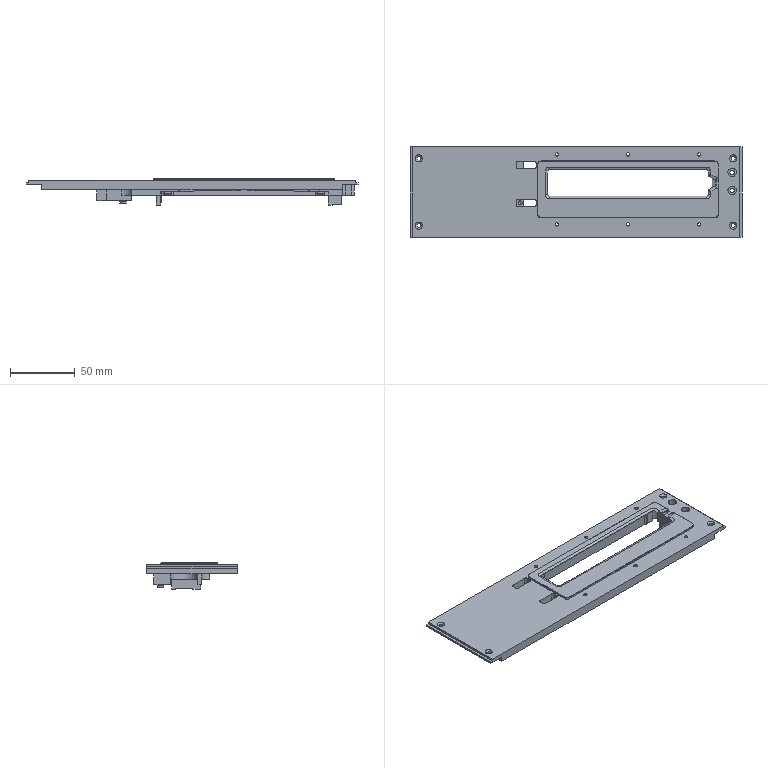NC program | NX | posted with a generic post | part box 256.6 x 70.3 x 20.422 mm
Lines 3316 to 4278 of 23702:
(CAVITY_MILL_COPY , TOOL : D6)
N6624 T06 M6
N6626 G54
N6628 G17 G0 G90 X20.674 Y0.131 S9500 M3
N6630 G43 Z30. H6
N6632 Z-0.118
N6634 G94 G1 Z-1.118 F1000.
N6636 G3 X21.494 Y0.695 R1.
N6638 G2 X21.913 Y1.34 R3. F1800.
N6640 G1 Y2.189
N6642 G3 X21.413 Y3.055 R1.
N6644 G1 X21.313 Y3.113
N6646 Z-0.118
N6648 G0 X20.598 Y-0.536 Z-0.522
N6650 G1 Z-1.522 F1000.
N6652 G3 X21.299 Y0.17 R1.
N6654 G2 X21.509 Y0.726 R3. F1800.
N6656 G1 Y1.349
N6658 G3 X21.009 Y2.215 R1.
N6660 G1 X20.909 Y2.272
N6662 Z-0.522
N6664 G0 X20.598 Y0.633 Z-1.022
N6666 G1 Z-2.022 F1000.
N6668 X20.698 Y0.691
N6670 G3 X21.198 Y1.557 R1.
N6672 G1 Y2.095 F1800.
N6674 G2 X21.057 Y2.607 R3.054
N6676 G3 X20.406 Y3.369 R1.
N6678 G1 Z-1.022
N6680 G0 X20.598 Y0.244 Z-1.522
N6682 G1 Z-2.522 F1000.
N6684 X20.698 Y0.301
N6686 G3 X21.198 Y1.167 R1.
N6688 G1 Y1.851 F1800.
N6690 G2 X20.937 Y2.437 R3.
N6692 G3 X20.2 Y3.106 R1.
N6694 G1 Z-1.522
N6696 G0 X20.598 Y0.244 Z-2.022
N6698 G1 Z-3.022 F1000.
N6700 X20.698 Y0.301
N6702 G3 X21.198 Y1.167 R1.
N6704 G1 Y1.851 F1800.
N6706 G2 X20.937 Y2.437 R3.
N6708 G3 X20.2 Y3.106 R1.
N6710 G1 Z-2.022
N6712 G0 X20.598 Y0.244 Z-2.522
N6714 G1 Z-3.522 F1000.
N6716 X20.698 Y0.301
N6718 G3 X21.198 Y1.167 R1.
N6720 G1 Y1.851 F1800.
N6722 G2 X20.937 Y2.437 R3.
N6724 G3 X20.2 Y3.106 R1.
N6726 G1 Z-2.522
N6728 G0 X20.598 Y0.244 Z-2.988
N6730 G1 Z-3.988 F1000.
N6732 X20.698 Y0.301
N6734 G3 X21.198 Y1.167 R1.
N6736 G1 Y1.851 F1800.
N6738 G2 X20.937 Y2.437 R3.
N6740 G3 X20.2 Y3.106 R1.
N6742 G1 Z-2.988
N6744 G0 X20.598 Y0.244 Z-3.455
N6746 G1 Z-4.455 F1000.
N6748 X20.698 Y0.301
N6750 G3 X21.198 Y1.167 R1.
N6752 G1 Y1.851 F1800.
N6754 G2 X20.937 Y2.437 R3.
N6756 G3 X20.2 Y3.106 R1.
N6758 G1 Z-3.455
N6760 G0 X20.598 Y0.244 Z-3.922
N6762 G1 Z-4.922 F1000.
N6764 X20.698 Y0.301
N6766 G3 X21.198 Y1.167 R1.
N6768 G1 Y1.851 F1800.
N6770 G2 X20.937 Y2.437 R3.
N6772 G3 X20.2 Y3.106 R1.
N6774 G1 Z-3.922
N6776 G0 X20.598 Y0.244 Z-4.388
N6778 G1 Z-5.388 F1000.
N6780 X20.698 Y0.301
N6782 G3 X21.198 Y1.167 R1.
N6784 G1 Y1.851 F1800.
N6786 G2 X20.937 Y2.437 R3.
N6788 G3 X20.2 Y3.106 R1.
N6790 G1 Z-4.388
N6792 G0 X20.598 Y0.244 Z-4.855
N6794 G1 Z-5.855 F1000.
N6796 X20.698 Y0.301
N6798 G3 X21.198 Y1.167 R1.
N6800 G1 Y1.851 F1800.
N6802 G2 X20.937 Y2.437 R3.
N6804 G3 X20.2 Y3.106 R1.
N6806 G1 Z-4.855
N6808 G0 X20.598 Y0.244 Z-5.322
N6810 G1 Z-6.322 F1000.
N6812 X20.698 Y0.301
N6814 G3 X21.198 Y1.167 R1.
N6816 G1 Y1.851 F1800.
N6818 G2 X20.937 Y2.437 R3.
N6820 G3 X20.2 Y3.106 R1.
N6822 G1 Z-5.322
N6824 G0 X20.598 Y0.244 Z-5.788
N6826 G1 Z-6.788 F1000.
N6828 X20.698 Y0.301
N6830 G3 X21.198 Y1.167 R1.
N6832 G1 Y1.851 F1800.
N6834 G2 X20.937 Y2.437 R3.
N6836 G3 X20.2 Y3.106 R1.
N6838 G1 Z-5.788
N6840 G0 X20.598 Y0.244 Z-6.255
N6842 G1 Z-7.255 F1000.
N6844 X20.698 Y0.301
N6846 G3 X21.198 Y1.167 R1.
N6848 G1 Y1.851 F1800.
N6850 G2 X20.937 Y2.437 R3.
N6852 G3 X20.2 Y3.106 R1.
N6854 G1 Z-6.255
N6856 G0 X20.598 Y0.244 Z-6.722
N6858 G1 Z-7.722 F1000.
N6860 X20.698 Y0.301
N6862 G3 X21.198 Y1.167 R1.
N6864 G1 Y1.851 F1800.
N6866 G2 X20.937 Y2.437 R3.
N6868 G3 X20.2 Y3.106 R1.
N6870 G1 Z-6.722
N6872 G0 X20.598 Y0.244 Z-7.216
N6874 G1 Z-8.216 F1000.
N6876 X20.698 Y0.301
N6878 G3 X21.198 Y1.167 R1.
N6880 G1 Y1.851 F1800.
N6882 G2 X20.937 Y2.437 R3.
N6884 G3 X20.2 Y3.106 R1.
N6886 G1 Z-7.216
N6888 G0 X20.598 Y0.244 Z-7.71
N6890 G1 Z-8.71 F1000.
N6892 X20.698 Y0.301
N6894 G3 X21.198 Y1.167 R1.
N6896 G1 Y1.851 F1800.
N6898 G2 X20.937 Y2.437 R3.
N6900 G3 X20.2 Y3.106 R1.
N6902 G1 Z-7.71
N6904 G0 X20.598 Y0.244 Z-8.204
N6906 G1 Z-9.204 F1000.
N6908 X20.698 Y0.301
N6910 G3 X21.198 Y1.167 R1.
N6912 G1 Y1.851 F1800.
N6914 G2 X20.937 Y2.437 R3.
N6916 G3 X20.2 Y3.106 R1.
N6918 G1 Z-8.204
N6920 G0 X20.598 Y0.244 Z-8.698
N6922 G1 Z-9.698 F1000.
N6924 X20.698 Y0.301
N6926 G3 X21.198 Y1.167 R1.
N6928 G1 Y1.851 F1800.
N6930 G2 X20.937 Y2.437 R3.
N6932 G3 X20.2 Y3.106 R1.
N6934 G1 Z-8.698
N6936 G0 X20.598 Y0.244 Z-9.192
N6938 G1 Z-10.192 F1000.
N6940 X20.698 Y0.301
N6942 G3 X21.198 Y1.167 R1.
N6944 G1 Y1.851 F1800.
N6946 G2 X20.937 Y2.437 R3.
N6948 G3 X20.2 Y3.106 R1.
N6950 G1 Z-9.192
N6952 G0 X20.598 Y0.244 Z-9.687
N6954 G1 Z-10.687 F1000.
N6956 X20.698 Y0.301
N6958 G3 X21.198 Y1.167 R1.
N6960 G1 Y1.851 F1800.
N6962 G2 X20.937 Y2.437 R3.
N6964 G3 X20.2 Y3.106 R1.
N6966 G1 Z-9.687
N6968 G0 X17.701 Y-3.1 Z-10.019
N6970 G1 Z-11.019 F1000.
N6972 X17.713 Y-3.127
N6974 G3 X18.52 Y-3.717 R1.
N6976 G2 X21.198 Y-6.66 R3. F1800.
N6978 G1 Y-1.585
N6980 G3 X20.698 Y-0.719 R1.
N6982 G1 X20.598 Y-0.662
N6984 Z-10.019
N6986 G0 X17.701 Y-3.1 Z-10.27
N6988 G1 Z-11.27 F1000.
N6990 X17.713 Y-3.127
N6992 G3 X18.52 Y-3.717 R1.
N6994 G2 X21.198 Y-6.66 R3. F1800.
N6996 G1 Y-1.585
N6998 G3 X20.698 Y-0.719 R1.
N7000 G1 X20.598 Y-0.662
N7002 Z-10.27
N7004 G0 X17.701 Y-3.1 Z-10.522
N7006 G1 Z-11.522 F1000.
N7008 X17.713 Y-3.127
N7010 G3 X18.52 Y-3.717 R1.
N7012 G2 X21.198 Y-6.66 R3. F1800.
N7014 G1 Y-1.585
N7016 G3 X20.698 Y-0.719 R1.
N7018 G1 X20.598 Y-0.662
N7020 Z-10.522
N7022 G0 X17.701 Y-3.1 Z-10.925
N7024 G1 Z-11.925 F1000.
N7026 X17.713 Y-3.127
N7028 G3 X18.52 Y-3.717 R1.
N7030 G2 X21.198 Y-6.66 R3. F1800.
N7032 G1 Y-1.585
N7034 G3 X20.698 Y-0.719 R1.
N7036 G1 X20.598 Y-0.662
N7038 Z-10.925
N7040 G0 X17.701 Y-3.1 Z-11.419
N7042 G1 Z-12.419 F1000.
N7044 X17.713 Y-3.127
N7046 G3 X18.52 Y-3.717 R1.
N7048 G2 X21.198 Y-6.66 R3. F1800.
N7050 G1 Y-1.585
N7052 G3 X20.698 Y-0.719 R1.
N7054 G1 X20.598 Y-0.662
N7056 Z-11.419
N7058 G0 X17.701 Y-3.1 Z-11.912
N7060 G1 Z-12.912 F1000.
N7062 X17.713 Y-3.127
N7064 G3 X18.52 Y-3.717 R1.
N7066 G2 X21.198 Y-6.66 R3. F1800.
N7068 G1 Y-1.585
N7070 G3 X20.698 Y-0.719 R1.
N7072 G1 X20.598 Y-0.662
N7074 Z-11.912
N7076 G0 X17.701 Y-3.1 Z-12.405
N7078 G1 Z-13.405 F1000.
N7080 X17.713 Y-3.127
N7082 G3 X18.52 Y-3.717 R1.
N7084 G2 X21.198 Y-6.66 R3. F1800.
N7086 G1 Y-1.585
N7088 G3 X20.698 Y-0.719 R1.
N7090 G1 X20.598 Y-0.662
N7092 Z-12.405
N7094 G0 X17.701 Y-3.1 Z-12.899
N7096 G1 Z-13.899 F1000.
N7098 X17.713 Y-3.127
N7100 G3 X18.52 Y-3.717 R1.
N7102 G2 X21.198 Y-6.66 R3. F1800.
N7104 G1 Y-1.585
N7106 G3 X20.698 Y-0.719 R1.
N7108 G1 X20.598 Y-0.662
N7110 Z-12.899
N7112 G0 X17.701 Y-3.1 Z-13.392
N7114 G1 Z-14.392 F1000.
N7116 X17.713 Y-3.127
N7118 G3 X18.52 Y-3.717 R1.
N7120 G2 X21.198 Y-6.66 R3. F1800.
N7122 G1 Y-1.585
N7124 G3 X20.698 Y-0.719 R1.
N7126 G1 X20.598 Y-0.662
N7128 Z-13.392
N7130 G0 X17.701 Y-3.1 Z-13.885
N7132 G1 Z-14.885 F1000.
N7134 X17.713 Y-3.127
N7136 G3 X18.52 Y-3.717 R1.
N7138 G2 X21.198 Y-6.66 R3. F1800.
N7140 G1 Y-1.585
N7142 G3 X20.698 Y-0.719 R1.
N7144 G1 X20.598 Y-0.662
N7146 Z-13.885
N7148 G0 X17.701 Y-3.1 Z-14.378
N7150 G1 Z-15.378 F1000.
N7152 X17.713 Y-3.127
N7154 G3 X18.52 Y-3.717 R1.
N7156 G2 X21.198 Y-6.66 R3. F1800.
N7158 G1 Y-1.585
N7160 G3 X20.698 Y-0.719 R1.
N7162 G1 X20.598 Y-0.662
N7164 Z-14.378
N7166 G0 X17.701 Y-3.1 Z-14.872
N7168 G1 Z-15.872 F1000.
N7170 X17.713 Y-3.127
N7172 G3 X18.52 Y-3.717 R1.
N7174 G2 X21.198 Y-6.66 R3. F1800.
N7176 G1 Y-1.585
N7178 G3 X20.698 Y-0.719 R1.
N7180 G1 X20.598 Y-0.662
N7182 Z-14.872
N7184 G0 X17.701 Y-3.1 Z-14.922
N7186 G1 Z-15.922 F1000.
N7188 X17.713 Y-3.127
N7190 G3 X18.52 Y-3.717 R1.
N7192 G2 X21.198 Y-6.66 R3. F1800.
N7194 G1 Y-1.585
N7196 G3 X20.698 Y-0.719 R1.
N7198 G1 X20.598 Y-0.662
N7200 Z-14.922
N7202 G0 X17.701 Y-3.1 Z-15.372
N7204 G1 Z-16.372 F1000.
N7206 X17.713 Y-3.127
N7208 G3 X18.52 Y-3.717 R1.
N7210 G2 X21.198 Y-6.66 R3. F1800.
N7212 G1 Y-1.585
N7214 G3 X20.698 Y-0.719 R1.
N7216 G1 X20.598 Y-0.662
N7218 Z-15.372
N7220 G0 X17.701 Y-3.1 Z-15.822
N7222 G1 Z-16.822 F1000.
N7224 X17.713 Y-3.127
N7226 G3 X18.52 Y-3.717 R1.
N7228 G2 X21.198 Y-6.66 R3. F1800.
N7230 G1 Y-1.585
N7232 G3 X20.698 Y-0.719 R1.
N7234 G1 X20.598 Y-0.662
N7236 Z-15.822
N7238 G0 X17.701 Y-3.1 Z-16.322
N7240 G1 Z-17.322 F1000.
N7242 X17.713 Y-3.127
N7244 G3 X18.52 Y-3.717 R1.
N7246 G2 X21.198 Y-6.66 R3. F1800.
N7248 G1 Y-1.585
N7250 G3 X20.698 Y-0.719 R1.
N7252 G1 X20.598 Y-0.662
N7254 Z-16.322
N7256 G0 X17.701 Y-3.1 Z-16.822
N7258 G1 Z-17.822 F1000.
N7260 X17.713 Y-3.127
N7262 G3 X18.52 Y-3.717 R1.
N7264 G2 X21.198 Y-6.66 R3. F1800.
N7266 G1 Y-1.585
N7268 G3 X20.698 Y-0.719 R1.
N7270 G1 X20.598 Y-0.662
N7272 Z-16.822
N7274 G0 X17.701 Y-3.1 Z-17.322
N7276 G1 Z-18.322 F1000.
N7278 X17.713 Y-3.127
N7280 G3 X18.52 Y-3.717 R1.
N7282 G2 X21.198 Y-6.66 R3. F1800.
N7284 G1 Y-1.585
N7286 G3 X20.698 Y-0.719 R1.
N7288 G1 X20.598 Y-0.662
N7290 Z-17.322
N7292 G0 X17.701 Y-3.1 Z-17.822
N7294 G1 Z-18.822 F1000.
N7296 X17.713 Y-3.127
N7298 G3 X18.52 Y-3.717 R1.
N7300 G2 X21.198 Y-6.66 R3. F1800.
N7302 G1 Y-1.585
N7304 G3 X20.698 Y-0.719 R1.
N7306 G1 X20.598 Y-0.662
N7308 Z-17.822
N7310 G0 X17.701 Y-3.1 Z-18.322
N7312 G1 Z-19.322 F1000.
N7314 X17.713 Y-3.127
N7316 G3 X18.52 Y-3.717 R1.
N7318 G2 X21.198 Y-6.66 R3. F1800.
N7320 G1 Y-1.585
N7322 G3 X20.698 Y-0.719 R1.
N7324 G1 X20.598 Y-0.662
N7326 Z-18.322
N7328 G0 Z30.
N7330 Y0.244
N7332 Z-10.019
N7334 G1 Z-11.019 F1000.
N7336 X20.698 Y0.301
N7338 G3 X21.198 Y1.167 R1.
N7340 G1 Y1.851 F1800.
N7342 G2 X20.937 Y2.437 R3.
N7344 G3 X20.2 Y3.106 R1.
N7346 G1 Z-10.019
N7348 G0 X20.598 Y0.244 Z-10.27
N7350 G1 Z-11.27 F1000.
N7352 X20.698 Y0.301
N7354 G3 X21.198 Y1.167 R1.
N7356 G1 Y1.851 F1800.
N7358 G2 X20.937 Y2.437 R3.
N7360 G3 X20.2 Y3.106 R1.
N7362 G1 Z-10.27
N7364 G0 X20.598 Y0.244 Z-10.522
N7366 G1 Z-11.522 F1000.
N7368 X20.698 Y0.301
N7370 G3 X21.198 Y1.167 R1.
N7372 G1 Y1.851 F1800.
N7374 G2 X20.937 Y2.437 R3.
N7376 G3 X20.2 Y3.106 R1.
N7378 G1 Z-10.522
N7380 G0 X20.598 Y0.244 Z-10.925
N7382 G1 Z-11.925 F1000.
N7384 X20.698 Y0.301
N7386 G3 X21.198 Y1.167 R1.
N7388 G1 Y1.851 F1800.
N7390 G2 X20.937 Y2.437 R3.
N7392 G3 X20.2 Y3.106 R1.
N7394 G1 Z-10.925
N7396 G0 X20.598 Y0.244 Z-11.419
N7398 G1 Z-12.419 F1000.
N7400 X20.698 Y0.301
N7402 G3 X21.198 Y1.167 R1.
N7404 G1 Y1.851 F1800.
N7406 G2 X20.937 Y2.437 R3.
N7408 G3 X20.2 Y3.106 R1.
N7410 G1 Z-11.419
N7412 G0 X20.598 Y0.244 Z-11.912
N7414 G1 Z-12.912 F1000.
N7416 X20.698 Y0.301
N7418 G3 X21.198 Y1.167 R1.
N7420 G1 Y1.851 F1800.
N7422 G2 X20.937 Y2.437 R3.
N7424 G3 X20.2 Y3.106 R1.
N7426 G1 Z-11.912
N7428 G0 X20.598 Y0.244 Z-12.405
N7430 G1 Z-13.405 F1000.
N7432 X20.698 Y0.301
N7434 G3 X21.198 Y1.167 R1.
N7436 G1 Y1.851 F1800.
N7438 G2 X20.937 Y2.437 R3.
N7440 G3 X20.2 Y3.106 R1.
N7442 G1 Z-12.405
N7444 G0 X20.598 Y0.244 Z-12.899
N7446 G1 Z-13.899 F1000.
N7448 X20.698 Y0.301
N7450 G3 X21.198 Y1.167 R1.
N7452 G1 Y1.851 F1800.
N7454 G2 X20.937 Y2.437 R3.
N7456 G3 X20.2 Y3.106 R1.
N7458 G1 Z-12.899
N7460 G0 X20.598 Y0.244 Z-13.392
N7462 G1 Z-14.392 F1000.
N7464 X20.698 Y0.301
N7466 G3 X21.198 Y1.167 R1.
N7468 G1 Y1.851 F1800.
N7470 G2 X20.937 Y2.437 R3.
N7472 G3 X20.2 Y3.106 R1.
N7474 G1 Z-13.392
N7476 G0 X20.598 Y0.244 Z-13.885
N7478 G1 Z-14.885 F1000.
N7480 X20.698 Y0.301
N7482 G3 X21.198 Y1.167 R1.
N7484 G1 Y1.851 F1800.
N7486 G2 X20.937 Y2.437 R3.
N7488 G3 X20.2 Y3.106 R1.
N7490 G1 Z-13.885
N7492 G0 X20.598 Y0.244 Z-14.378
N7494 G1 Z-15.378 F1000.
N7496 X20.698 Y0.301
N7498 G3 X21.198 Y1.167 R1.
N7500 G1 Y1.851 F1800.
N7502 G2 X20.937 Y2.437 R3.
N7504 G3 X20.2 Y3.106 R1.
N7506 G1 Z-14.378
N7508 G0 X20.598 Y0.244 Z-14.872
N7510 G1 Z-15.872 F1000.
N7512 X20.698 Y0.301
N7514 G3 X21.198 Y1.167 R1.
N7516 G1 Y1.851 F1800.
N7518 G2 X20.937 Y2.437 R3.
N7520 G3 X20.2 Y3.106 R1.
N7522 G1 Z-14.872
N7524 G0 X20.598 Y0.244 Z-14.922
N7526 G1 Z-15.922 F1000.
N7528 X20.698 Y0.301
N7530 G3 X21.198 Y1.167 R1.
N7532 G1 Y1.851 F1800.
N7534 G2 X20.937 Y2.437 R3.
N7536 G3 X20.2 Y3.106 R1.
N7538 G1 Z-14.922
N7540 G0 X20.598 Y0.244 Z-15.372
N7542 G1 Z-16.372 F1000.
N7544 X20.698 Y0.301
N7546 G3 X21.198 Y1.167 R1.
N7548 G1 Y1.851 F1800.
N7550 G2 X20.937 Y2.437 R3.
N7552 G3 X20.2 Y3.106 R1.
N7554 G1 Z-15.372
N7556 G0 X20.598 Y0.244 Z-15.822
N7558 G1 Z-16.822 F1000.
N7560 X20.698 Y0.301
N7562 G3 X21.198 Y1.167 R1.
N7564 G1 Y1.851 F1800.
N7566 G2 X20.937 Y2.437 R3.
N7568 G3 X20.2 Y3.106 R1.
N7570 G1 Z-15.822
N7572 G0 X20.598 Y0.244 Z-16.322
N7574 G1 Z-17.322 F1000.
N7576 X20.698 Y0.301
N7578 G3 X21.198 Y1.167 R1.
N7580 G1 Y1.851 F1800.
N7582 G2 X20.937 Y2.437 R3.
N7584 G3 X20.2 Y3.106 R1.
N7586 G1 Z-16.322
N7588 G0 X20.598 Y0.244 Z-16.822
N7590 G1 Z-17.822 F1000.
N7592 X20.698 Y0.301
N7594 G3 X21.198 Y1.167 R1.
N7596 G1 Y1.851 F1800.
N7598 G2 X20.937 Y2.437 R3.
N7600 G3 X20.2 Y3.106 R1.
N7602 G1 Z-16.822
N7604 G0 X20.598 Y0.244 Z-17.322
N7606 G1 Z-18.322 F1000.
N7608 X20.698 Y0.301
N7610 G3 X21.198 Y1.167 R1.
N7612 G1 Y1.851 F1800.
N7614 G2 X20.937 Y2.437 R3.
N7616 G3 X20.2 Y3.106 R1.
N7618 G1 Z-17.322
N7620 G0 X20.598 Y0.244 Z-17.822
N7622 G1 Z-18.822 F1000.
N7624 X20.698 Y0.301
N7626 G3 X21.198 Y1.167 R1.
N7628 G1 Y1.851 F1800.
N7630 G2 X20.937 Y2.437 R3.
N7632 G3 X20.2 Y3.106 R1.
N7634 G1 Z-17.822
N7636 G0 X20.598 Y0.244 Z-18.322
N7638 G1 Z-19.322 F1000.
N7640 X20.698 Y0.301
N7642 G3 X21.198 Y1.167 R1.
N7644 G1 Y1.851 F1800.
N7646 G2 X20.937 Y2.437 R3.
N7648 G3 X20.2 Y3.106 R1.
N7650 G1 Z-18.322
N7652 G0 Z30.
N7654 X21.313 Y8.887
N7656 Z-0.118
N7658 G1 Z-1.118 F1000.
N7660 X21.413 Y8.945
N7662 G3 X21.913 Y9.811 R1.
N7664 G1 Y10.66 F1800.
N7666 G2 X21.494 Y11.305 R3.
N7668 G3 X20.674 Y11.869 R1.
N7670 G1 Z-0.118
N7672 G0 X20.909 Y9.728 Z-0.522
N7674 G1 Z-1.522 F1000.
N7676 X21.009 Y9.785
N7678 G3 X21.509 Y10.651 R1.
N7680 G1 Y11.274 F1800.
N7682 G2 X21.299 Y11.83 R3.
N7684 G3 X20.598 Y12.536 R1.
N7686 G1 Z-0.522
N7688 G0 X20.406 Y8.601 Z-1.022
N7690 G1 Z-2.022 F1000.
N7692 X20.412 Y8.603
N7694 G3 X21.053 Y9.37 R1.
N7696 G2 X21.198 Y9.912 R3.175 F1800.
N7698 G1 Y10.472
N7700 G3 X20.698 Y11.338 R1.
N7702 G1 X20.598 Y11.396
N7704 Z-1.022
N7706 G0 X20.2 Y8.894 Z-1.522
N7708 G1 Z-2.522 F1000.
N7710 G3 X20.937 Y9.563 R1.
N7712 G2 X21.198 Y10.149 R3. F1800.
N7714 G1 Y10.833
N7716 G3 X20.698 Y11.699 R1.
N7718 G1 X20.598 Y11.756
N7720 Z-1.522
N7722 G0 X20.2 Y8.894 Z-2.022
N7724 G1 Z-3.022 F1000.
N7726 G3 X20.937 Y9.563 R1.
N7728 G2 X21.198 Y10.149 R3. F1800.
N7730 G1 Y10.833
N7732 G3 X20.698 Y11.699 R1.
N7734 G1 X20.598 Y11.756
N7736 Z-2.022
N7738 G0 X20.2 Y8.894 Z-2.522
N7740 G1 Z-3.522 F1000.
N7742 G3 X20.937 Y9.563 R1.
N7744 G2 X21.198 Y10.149 R3. F1800.
N7746 G1 Y10.833
N7748 G3 X20.698 Y11.699 R1.
N7750 G1 X20.598 Y11.756
N7752 Z-2.522
N7754 G0 X20.2 Y8.894 Z-2.988
N7756 G1 Z-3.988 F1000.
N7758 G3 X20.937 Y9.563 R1.
N7760 G2 X21.198 Y10.149 R3. F1800.
N7762 G1 Y10.833
N7764 G3 X20.698 Y11.699 R1.
N7766 G1 X20.598 Y11.756
N7768 Z-2.988
N7770 G0 X20.2 Y8.894 Z-3.455
N7772 G1 Z-4.455 F1000.
N7774 G3 X20.937 Y9.563 R1.
N7776 G2 X21.198 Y10.149 R3. F1800.
N7778 G1 Y10.833
N7780 G3 X20.698 Y11.699 R1.
N7782 G1 X20.598 Y11.756
N7784 Z-3.455
N7786 G0 X20.2 Y8.894 Z-3.922
N7788 G1 Z-4.922 F1000.
N7790 G3 X20.937 Y9.563 R1.
N7792 G2 X21.198 Y10.149 R3. F1800.
N7794 G1 Y10.833
N7796 G3 X20.698 Y11.699 R1.
N7798 G1 X20.598 Y11.756
N7800 Z-3.922
N7802 G0 X20.2 Y8.894 Z-4.388
N7804 G1 Z-5.388 F1000.
N7806 G3 X20.937 Y9.563 R1.
N7808 G2 X21.198 Y10.149 R3. F1800.
N7810 G1 Y10.833
N7812 G3 X20.698 Y11.699 R1.
N7814 G1 X20.598 Y11.756
N7816 Z-4.388
N7818 G0 X20.2 Y8.894 Z-4.855
N7820 G1 Z-5.855 F1000.
N7822 G3 X20.937 Y9.563 R1.
N7824 G2 X21.198 Y10.149 R3. F1800.
N7826 G1 Y10.833
N7828 G3 X20.698 Y11.699 R1.
N7830 G1 X20.598 Y11.756
N7832 Z-4.855
N7834 G0 X20.2 Y8.894 Z-5.322
N7836 G1 Z-6.322 F1000.
N7838 G3 X20.937 Y9.563 R1.
N7840 G2 X21.198 Y10.149 R3. F1800.
N7842 G1 Y10.833
N7844 G3 X20.698 Y11.699 R1.
N7846 G1 X20.598 Y11.756
N7848 Z-5.322
N7850 G0 X20.2 Y8.894 Z-5.788
N7852 G1 Z-6.788 F1000.
N7854 G3 X20.937 Y9.563 R1.
N7856 G2 X21.198 Y10.149 R3. F1800.
N7858 G1 Y10.833
N7860 G3 X20.698 Y11.699 R1.
N7862 G1 X20.598 Y11.756
N7864 Z-5.788
N7866 G0 X20.2 Y8.894 Z-6.255
N7868 G1 Z-7.255 F1000.
N7870 G3 X20.937 Y9.563 R1.
N7872 G2 X21.198 Y10.149 R3. F1800.
N7874 G1 Y10.833
N7876 G3 X20.698 Y11.699 R1.
N7878 G1 X20.598 Y11.756
N7880 Z-6.255
N7882 G0 X20.2 Y8.894 Z-6.722
N7884 G1 Z-7.722 F1000.
N7886 G3 X20.937 Y9.563 R1.
N7888 G2 X21.198 Y10.149 R3. F1800.
N7890 G1 Y10.833
N7892 G3 X20.698 Y11.699 R1.
N7894 G1 X20.598 Y11.756
N7896 Z-6.722
N7898 G0 X20.2 Y8.894 Z-7.216
N7900 G1 Z-8.216 F1000.
N7902 G3 X20.937 Y9.563 R1.
N7904 G2 X21.198 Y10.149 R3. F1800.
N7906 G1 Y10.833
N7908 G3 X20.698 Y11.699 R1.
N7910 G1 X20.598 Y11.756
N7912 Z-7.216
N7914 G0 X20.2 Y8.894 Z-7.71
N7916 G1 Z-8.71 F1000.
N7918 G3 X20.937 Y9.563 R1.
N7920 G2 X21.198 Y10.149 R3. F1800.
N7922 G1 Y10.833
N7924 G3 X20.698 Y11.699 R1.
N7926 G1 X20.598 Y11.756
N7928 Z-7.71
N7930 G0 X20.2 Y8.894 Z-8.204
N7932 G1 Z-9.204 F1000.
N7934 G3 X20.937 Y9.563 R1.
N7936 G2 X21.198 Y10.149 R3. F1800.
N7938 G1 Y10.833
N7940 G3 X20.698 Y11.699 R1.
N7942 G1 X20.598 Y11.756
N7944 Z-8.204
N7946 G0 X20.2 Y8.894 Z-8.698
N7948 G1 Z-9.698 F1000.
N7950 G3 X20.937 Y9.563 R1.
N7952 G2 X21.198 Y10.149 R3. F1800.
N7954 G1 Y10.833
N7956 G3 X20.698 Y11.699 R1.
N7958 G1 X20.598 Y11.756
N7960 Z-8.698
N7962 G0 X20.2 Y8.894 Z-9.192
N7964 G1 Z-10.192 F1000.
N7966 G3 X20.937 Y9.563 R1.
N7968 G2 X21.198 Y10.149 R3. F1800.
N7970 G1 Y10.833
N7972 G3 X20.698 Y11.699 R1.
N7974 G1 X20.598 Y11.756
N7976 Z-9.192
N7978 G0 X20.2 Y8.894 Z-9.687
N7980 G1 Z-10.687 F1000.
N7982 G3 X20.937 Y9.563 R1.
N7984 G2 X21.198 Y10.149 R3. F1800.
N7986 G1 Y10.833
N7988 G3 X20.698 Y11.699 R1.
N7990 G1 X20.598 Y11.756
N7992 Z-9.687
N7994 G0 X20.2 Y8.894 Z-10.019
N7996 G1 Z-11.019 F1000.
N7998 G3 X20.937 Y9.563 R1.
N8000 G2 X21.198 Y10.149 R3. F1800.
N8002 G1 Y10.833
N8004 G3 X20.698 Y11.699 R1.
N8006 G1 X20.598 Y11.756
N8008 Z-10.019
N8010 G0 X20.2 Y8.894 Z-10.27
N8012 G1 Z-11.27 F1000.
N8014 G3 X20.937 Y9.563 R1.
N8016 G2 X21.198 Y10.149 R3. F1800.
N8018 G1 Y10.833
N8020 G3 X20.698 Y11.699 R1.
N8022 G1 X20.598 Y11.756
N8024 Z-10.27
N8026 G0 X20.2 Y8.894 Z-10.522
N8028 G1 Z-11.522 F1000.
N8030 G3 X20.937 Y9.563 R1.
N8032 G2 X21.198 Y10.149 R3. F1800.
N8034 G1 Y10.833
N8036 G3 X20.698 Y11.699 R1.
N8038 G1 X20.598 Y11.756
N8040 Z-10.522
N8042 G0 X20.2 Y8.894 Z-10.925
N8044 G1 Z-11.925 F1000.
N8046 G3 X20.937 Y9.563 R1.
N8048 G2 X21.198 Y10.149 R3. F1800.
N8050 G1 Y10.833
N8052 G3 X20.698 Y11.699 R1.
N8054 G1 X20.598 Y11.756
N8056 Z-10.925
N8058 G0 X20.2 Y8.894 Z-11.419
N8060 G1 Z-12.419 F1000.
N8062 G3 X20.937 Y9.563 R1.
N8064 G2 X21.198 Y10.149 R3. F1800.
N8066 G1 Y10.833
N8068 G3 X20.698 Y11.699 R1.
N8070 G1 X20.598 Y11.756
N8072 Z-11.419
N8074 G0 X20.2 Y8.894 Z-11.912
N8076 G1 Z-12.912 F1000.
N8078 G3 X20.937 Y9.563 R1.
N8080 G2 X21.198 Y10.149 R3. F1800.
N8082 G1 Y10.833
N8084 G3 X20.698 Y11.699 R1.
N8086 G1 X20.598 Y11.756
N8088 Z-11.912
N8090 G0 X20.2 Y8.894 Z-12.405
N8092 G1 Z-13.405 F1000.
N8094 G3 X20.937 Y9.563 R1.
N8096 G2 X21.198 Y10.149 R3. F1800.
N8098 G1 Y10.833
N8100 G3 X20.698 Y11.699 R1.
N8102 G1 X20.598 Y11.756
N8104 Z-12.405
N8106 G0 X20.2 Y8.894 Z-12.899
N8108 G1 Z-13.899 F1000.
N8110 G3 X20.937 Y9.563 R1.
N8112 G2 X21.198 Y10.149 R3. F1800.
N8114 G1 Y10.833
N8116 G3 X20.698 Y11.699 R1.
N8118 G1 X20.598 Y11.756
N8120 Z-12.899
N8122 G0 X20.2 Y8.894 Z-13.392
N8124 G1 Z-14.392 F1000.
N8126 G3 X20.937 Y9.563 R1.
N8128 G2 X21.198 Y10.149 R3. F1800.
N8130 G1 Y10.833
N8132 G3 X20.698 Y11.699 R1.
N8134 G1 X20.598 Y11.756
N8136 Z-13.392
N8138 G0 X20.2 Y8.894 Z-13.885
N8140 G1 Z-14.885 F1000.
N8142 G3 X20.937 Y9.563 R1.
N8144 G2 X21.198 Y10.149 R3. F1800.
N8146 G1 Y10.833
N8148 G3 X20.698 Y11.699 R1.
N8150 G1 X20.598 Y11.756
N8152 Z-13.885
N8154 G0 X20.2 Y8.894 Z-14.378
N8156 G1 Z-15.378 F1000.
N8158 G3 X20.937 Y9.563 R1.
N8160 G2 X21.198 Y10.149 R3. F1800.
N8162 G1 Y10.833
N8164 G3 X20.698 Y11.699 R1.
N8166 G1 X20.598 Y11.756
N8168 Z-14.378
N8170 G0 X20.2 Y8.894 Z-14.872
N8172 G1 Z-15.872 F1000.
N8174 G3 X20.937 Y9.563 R1.
N8176 G2 X21.198 Y10.149 R3. F1800.
N8178 G1 Y10.833
N8180 G3 X20.698 Y11.699 R1.
N8182 G1 X20.598 Y11.756
N8184 Z-14.872
N8186 G0 X20.2 Y8.894 Z-14.922
N8188 G1 Z-15.922 F1000.
N8190 G3 X20.937 Y9.563 R1.
N8192 G2 X21.198 Y10.149 R3. F1800.
N8194 G1 Y10.833
N8196 G3 X20.698 Y11.699 R1.
N8198 G1 X20.598 Y11.756
N8200 Z-14.922
N8202 G0 X20.2 Y8.894 Z-15.372
N8204 G1 Z-16.372 F1000.
N8206 G3 X20.937 Y9.563 R1.
N8208 G2 X21.198 Y10.149 R3. F1800.
N8210 G1 Y10.833
N8212 G3 X20.698 Y11.699 R1.
N8214 G1 X20.598 Y11.756
N8216 Z-15.372
N8218 G0 X20.2 Y8.894 Z-15.822
N8220 G1 Z-16.822 F1000.
N8222 G3 X20.937 Y9.563 R1.
N8224 G2 X21.198 Y10.149 R3. F1800.
N8226 G1 Y10.833
N8228 G3 X20.698 Y11.699 R1.
N8230 G1 X20.598 Y11.756
N8232 Z-15.822
N8234 G0 X20.2 Y8.894 Z-16.322
N8236 G1 Z-17.322 F1000.
N8238 G3 X20.937 Y9.563 R1.
N8240 G2 X21.198 Y10.149 R3. F1800.
N8242 G1 Y10.833
N8244 G3 X20.698 Y11.699 R1.
N8246 G1 X20.598 Y11.756
N8248 Z-16.322
N8250 G0 X20.2 Y8.894 Z-16.822
N8252 G1 Z-17.822 F1000.
N8254 G3 X20.937 Y9.563 R1.
N8256 G2 X21.198 Y10.149 R3. F1800.
N8258 G1 Y10.833
N8260 G3 X20.698 Y11.699 R1.
N8262 G1 X20.598 Y11.756
N8264 Z-16.822
N8266 G0 X20.2 Y8.894 Z-17.322
N8268 G1 Z-18.322 F1000.
N8270 G3 X20.937 Y9.563 R1.
N8272 G2 X21.198 Y10.149 R3. F1800.
N8274 G1 Y10.833
N8276 G3 X20.698 Y11.699 R1.
N8278 G1 X20.598 Y11.756
N8280 Z-17.322
N8282 G0 X20.2 Y8.894 Z-17.822
N8284 G1 Z-18.822 F1000.
N8286 G3 X20.937 Y9.563 R1.
N8288 G2 X21.198 Y10.149 R3. F1800.
N8290 G1 Y10.833
N8292 G3 X20.698 Y11.699 R1.
N8294 G1 X20.598 Y11.756
N8296 Z-17.822
N8298 G0 X20.2 Y8.894 Z-18.322
N8300 G1 Z-19.322 F1000.
N8302 G3 X20.937 Y9.563 R1.
N8304 G2 X21.198 Y10.149 R3. F1800.
N8306 G1 Y10.833
N8308 G3 X20.698 Y11.699 R1.
N8310 G1 X20.598 Y11.756
N8312 Z-18.322
N8314 G0 Z30.
N8316 Y13.566
N8318 Z-7.216
N8320 G1 Z-8.216 F1000.
N8322 X20.698 Y13.623
N8324 G3 X21.198 Y14.489 R1.
N8326 G1 Y15.7 F1800.
N8328 G2 X21.371 Y16.706 R3.
N8330 G1 X18.981
N8332 G3 X18.115 Y16.206 R1.
N8334 G1 X18.058 Y16.106
N8336 Z-7.216
N8338 G0 X20.598 Y13.071 Z-7.71
N8340 G1 Z-8.71 F1000.
N8342 X20.698 Y13.129
N8344 G3 X21.198 Y13.995 R1.
N8346 G1 Y15.7 F1800.
N8348 G2 X21.242 Y16.212 R3.
N8350 G1 X18.981
N8352 G3 X18.115 Y15.712 R1.
N8354 G1 X18.058 Y15.612
N8356 Z-7.71
N8358 G0 X20.598 Y12.577 Z-8.204
N8360 G1 Z-9.204 F1000.
N8362 X20.698 Y12.635
N8364 G3 X21.198 Y13.501 R1.
N8366 G1 Y15.718 F1800.
N8368 X18.981
N8370 G3 X18.115 Y15.218 R1.
N8372 G1 X18.058 Y15.118
N8374 Z-8.204
N8376 G0 X20.598 Y12.561 Z-8.698
N8378 G1 Z-9.698 F1000.
N8380 X20.698 Y12.619
N8382 G3 X21.198 Y13.485 R1.
N8384 G1 Y15.7 F1800.
N8386 X18.988
N8388 G3 X18.122 Y15.2 R1.
N8390 G1 X18.064 Y15.1
N8392 Z-8.698
N8394 G0 X20.598 Y12.561 Z-9.192
N8396 G1 Z-10.192 F1000.
N8398 X20.698 Y12.618
N8400 G3 X21.198 Y13.484 R1.
N8402 G1 Y15.7 F1800.
N8404 X18.988
N8406 G3 X18.122 Y15.2 R1.
N8408 G1 X18.064 Y15.1
N8410 Z-9.192
N8412 G0 X20.598 Y12.561 Z-9.687
N8414 G1 Z-10.687 F1000.
N8416 X20.698 Y12.618
N8418 G3 X21.198 Y13.484 R1.
N8420 G1 Y15.7 F1800.
N8422 X18.987
N8424 G3 X18.121 Y15.2 R1.
N8426 G1 X18.063 Y15.1
N8428 Z-9.687
N8430 G0 X20.598 Y12.561 Z-10.019
N8432 G1 Z-11.019 F1000.
N8434 X20.698 Y12.618
N8436 G3 X21.198 Y13.484 R1.
N8438 G1 Y15.7 F1800.
N8440 X18.987
N8442 G3 X18.121 Y15.2 R1.
N8444 G1 X18.063 Y15.1
N8446 Z-10.019
N8448 G0 X20.598 Y12.561 Z-10.27
N8450 G1 Z-11.27 F1000.
N8452 X20.698 Y12.618
N8454 G3 X21.198 Y13.484 R1.
N8456 G1 Y15.7 F1800.
N8458 X18.987
N8460 G3 X18.121 Y15.2 R1.
N8462 G1 X18.063 Y15.1
N8464 Z-10.27
N8466 G0 X20.598 Y12.561 Z-10.522
N8468 G1 Z-11.522 F1000.
N8470 X20.698 Y12.618
N8472 G3 X21.198 Y13.484 R1.
N8474 G1 Y15.7 F1800.
N8476 X18.986
N8478 G3 X18.12 Y15.2 R1.
N8480 G1 X18.063 Y15.1
N8482 Z-10.522
N8484 G0 X20.598 Y12.56 Z-10.925
N8486 G1 Z-11.925 F1000.
N8488 X20.698 Y12.618
N8490 G3 X21.198 Y13.484 R1.
N8492 G1 Y15.7 F1800.
N8494 X18.986
N8496 G3 X18.12 Y15.2 R1.
N8498 G1 X18.062 Y15.1
N8500 Z-10.925
N8502 G0 X20.598 Y12.56 Z-11.419
N8504 G1 Z-12.419 F1000.
N8506 X20.698 Y12.618
N8508 G3 X21.198 Y13.484 R1.
N8510 G1 Y15.7 F1800.
N8512 X18.986
N8514 G3 X18.12 Y15.2 R1.
N8516 G1 X18.062 Y15.1
N8518 Z-11.419
N8520 G0 X20.598 Y12.56 Z-11.912
N8522 G1 Z-12.912 F1000.
N8524 X20.698 Y12.618
N8526 G3 X21.198 Y13.484 R1.
N8528 G1 Y15.7 F1800.
N8530 X18.985
N8532 G3 X18.119 Y15.2 R1.
N8534 G1 X18.061 Y15.1
N8536 Z-11.912
N8538 G0 X20.598 Y12.56 Z-12.405
N8540 G1 Z-13.405 F1000.
N8542 X20.698 Y12.618